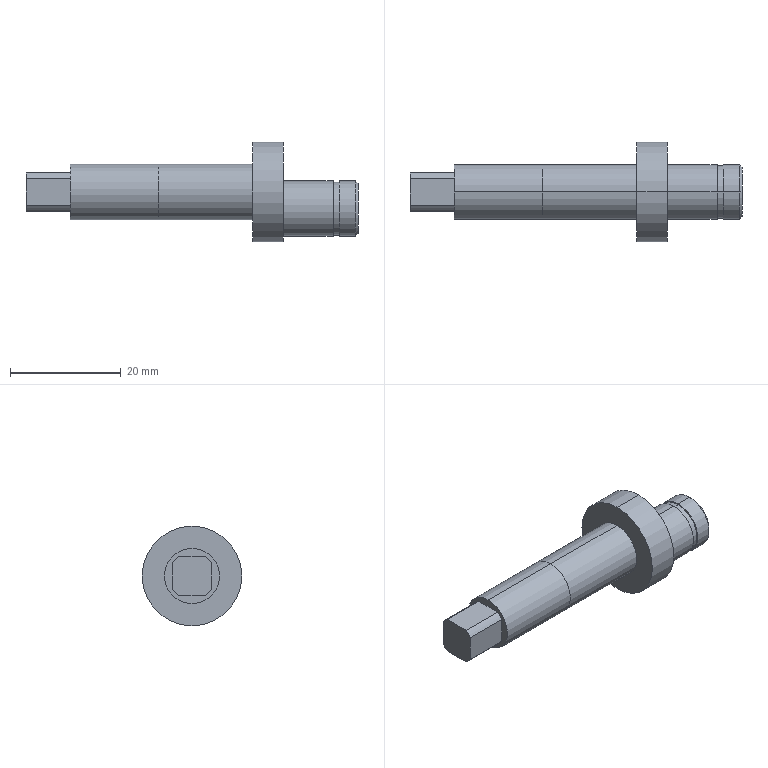Part | SolidWorks | features ICE 6, Chamfer 1, Extrusion 1 | 2 solids | 31 faces | box 60 x 18 x 18 mm | volume 5416 mm3 | cylinder 16 | plane 13 | cone 2 | commonest cylinder face diameters 10 x8 8.5 x4 9.6 x2 18 x2
STEP:
#1=CARTESIAN_POINT('',(-17.,0.,5.));
#2=VERTEX_POINT('',#1);
#3=CARTESIAN_POINT('',(-17.,0.,-5.));
#4=VERTEX_POINT('',#3);
#5=CARTESIAN_POINT('',(-17.,0.,0.));
#6=DIRECTION('',(-1.,0.,0.));
#7=DIRECTION('',(0.,0.,1.));
#8=AXIS2_PLACEMENT_3D('',#5,#6,#7);
#9=CIRCLE('',#8,5.);
#10=EDGE_CURVE('',#2,#4,#9,.T.);
#11=ORIENTED_EDGE('',*,*,#10,.F.);
#12=CARTESIAN_POINT('',(0.,0.,5.));
#13=VERTEX_POINT('',#12);
#14=CARTESIAN_POINT('',(-17.,0.,5.));
#15=DIRECTION('',(1.,0.,0.));
#16=VECTOR('',#15,1000.);
#17=LINE('',#14,#16);
#18=EDGE_CURVE('',#2,#13,#17,.T.);
#19=ORIENTED_EDGE('',*,*,#18,.T.);
#20=CARTESIAN_POINT('',(0.,0.,-5.));
#21=VERTEX_POINT('',#20);
#22=CARTESIAN_POINT('',(0.,0.,0.));
#23=DIRECTION('',(-1.,0.,0.));
#24=DIRECTION('',(0.,0.,1.));
#25=AXIS2_PLACEMENT_3D('',#22,#23,#24);
#26=CIRCLE('',#25,5.);
#27=EDGE_CURVE('',#13,#21,#26,.T.);
#28=ORIENTED_EDGE('',*,*,#27,.T.);
#29=CARTESIAN_POINT('',(-17.,0.,-5.));
#30=DIRECTION('',(1.,0.,0.));
#31=VECTOR('',#30,1000.);
#32=LINE('',#29,#31);
#33=EDGE_CURVE('',#4,#21,#32,.T.);
#34=ORIENTED_EDGE('',*,*,#33,.F.);
#35=EDGE_LOOP('',(#11,#19,#28,#34));
#36=FACE_OUTER_BOUND('',#35,.T.);
#37=CARTESIAN_POINT('',(-17.,0.,0.));
#38=DIRECTION('',(1.,0.,0.));
#39=DIRECTION('',(0.,0.,-1.));
#40=AXIS2_PLACEMENT_3D('',#37,#38,#39);
#41=CYLINDRICAL_SURFACE('',#40,5.);
#42=ADVANCED_FACE('',(#36),#41,.T.);
#43=CARTESIAN_POINT('',(19.,0.,-7.5));
#44=VERTEX_POINT('',#43);
#45=CARTESIAN_POINT('',(19.,0.,1.5));
#46=VERTEX_POINT('',#45);
#47=CARTESIAN_POINT('',(19.,0.,-3.));
#48=DIRECTION('',(1.,0.,0.));
#49=DIRECTION('',(0.,0.,-1.));
#50=AXIS2_PLACEMENT_3D('',#47,#48,#49);
#51=CIRCLE('',#50,4.5);
#52=EDGE_CURVE('',#44,#46,#51,.T.);
#53=ORIENTED_EDGE('',*,*,#52,.F.);
#54=CARTESIAN_POINT('',(18.5,0.,-8.));
#55=VERTEX_POINT('',#54);
#56=CARTESIAN_POINT('',(19.,0.,-7.5));
#57=DIRECTION('',(-0.7071,0.,-0.7071));
#58=VECTOR('',#57,1000.);
#59=LINE('',#56,#58);
#60=EDGE_CURVE('',#44,#55,#59,.T.);
#61=ORIENTED_EDGE('',*,*,#60,.T.);
#62=CARTESIAN_POINT('',(18.5,0.,2.));
#63=VERTEX_POINT('',#62);
#64=CARTESIAN_POINT('',(18.5,0.,-3.));
#65=DIRECTION('',(-1.,0.,0.));
#66=DIRECTION('',(0.,0.,-1.));
#67=AXIS2_PLACEMENT_3D('',#64,#65,#66);
#68=CIRCLE('',#67,5.);
#69=EDGE_CURVE('',#63,#55,#68,.T.);
#70=ORIENTED_EDGE('',*,*,#69,.F.);
#71=CARTESIAN_POINT('',(19.,0.,1.5));
#72=DIRECTION('',(-0.7071,0.,0.7071));
#73=VECTOR('',#72,1000.);
#74=LINE('',#71,#73);
#75=EDGE_CURVE('',#46,#63,#74,.T.);
#76=ORIENTED_EDGE('',*,*,#75,.F.);
#77=EDGE_LOOP('',(#53,#61,#70,#76));
#78=FACE_OUTER_BOUND('',#77,.T.);
#79=CARTESIAN_POINT('',(19.,0.,-3.));
#80=DIRECTION('',(-1.,0.,0.));
#81=DIRECTION('',(0.,0.,1.));
#82=AXIS2_PLACEMENT_3D('',#79,#80,#81);
#83=CONICAL_SURFACE('',#82,4.5,0.7854);
#84=ADVANCED_FACE('',(#78),#83,.T.);
#85=ORIENTED_EDGE('',*,*,#69,.T.);
#86=CARTESIAN_POINT('',(15.6,0.,-8.));
#87=VERTEX_POINT('',#86);
#88=CARTESIAN_POINT('',(19.,0.,-8.));
#89=DIRECTION('',(-1.,0.,0.));
#90=VECTOR('',#89,1000.);
#91=LINE('',#88,#90);
#92=EDGE_CURVE('',#55,#87,#91,.T.);
#93=ORIENTED_EDGE('',*,*,#92,.T.);
#94=CARTESIAN_POINT('',(15.6,0.,2.));
#95=VERTEX_POINT('',#94);
#96=CARTESIAN_POINT('',(15.6,0.,-3.));
#97=DIRECTION('',(1.,0.,0.));
#98=DIRECTION('',(0.,0.,-1.));
#99=AXIS2_PLACEMENT_3D('',#96,#97,#98);
#100=CIRCLE('',#99,5.);
#101=EDGE_CURVE('',#87,#95,#100,.T.);
#102=ORIENTED_EDGE('',*,*,#101,.T.);
#103=CARTESIAN_POINT('',(19.,0.,2.));
#104=DIRECTION('',(-1.,0.,0.));
#105=VECTOR('',#104,1000.);
#106=LINE('',#103,#105);
#107=EDGE_CURVE('',#63,#95,#106,.T.);
#108=ORIENTED_EDGE('',*,*,#107,.F.);
#109=EDGE_LOOP('',(#85,#93,#102,#108));
#110=FACE_OUTER_BOUND('',#109,.T.);
#111=CARTESIAN_POINT('',(19.,0.,-3.));
#112=DIRECTION('',(-1.,0.,0.));
#113=DIRECTION('',(0.,0.,1.));
#114=AXIS2_PLACEMENT_3D('',#111,#112,#113);
#115=CYLINDRICAL_SURFACE('',#114,5.);
#116=ADVANCED_FACE('',(#110),#115,.T.);
#117=CARTESIAN_POINT('',(15.6,0.,-7.8));
#118=VERTEX_POINT('',#117);
#119=CARTESIAN_POINT('',(15.6,0.,1.8));
#120=VERTEX_POINT('',#119);
#121=CARTESIAN_POINT('',(15.6,0.,-3.));
#122=DIRECTION('',(1.,0.,0.));
#123=DIRECTION('',(0.,0.,-1.));
#124=AXIS2_PLACEMENT_3D('',#121,#122,#123);
#125=CIRCLE('',#124,4.8);
#126=EDGE_CURVE('',#118,#120,#125,.T.);
#127=ORIENTED_EDGE('',*,*,#126,.F.);
#128=CARTESIAN_POINT('',(14.5,0.,-7.8));
#129=VERTEX_POINT('',#128);
#130=CARTESIAN_POINT('',(15.6,0.,-7.8));
#131=DIRECTION('',(-1.,0.,0.));
#132=VECTOR('',#131,1000.);
#133=LINE('',#130,#132);
#134=EDGE_CURVE('',#118,#129,#133,.T.);
#135=ORIENTED_EDGE('',*,*,#134,.T.);
#136=CARTESIAN_POINT('',(14.5,0.,1.8));
#137=VERTEX_POINT('',#136);
#138=CARTESIAN_POINT('',(14.5,0.,-3.));
#139=DIRECTION('',(1.,0.,0.));
#140=DIRECTION('',(0.,0.,-1.));
#141=AXIS2_PLACEMENT_3D('',#138,#139,#140);
#142=CIRCLE('',#141,4.8);
#143=EDGE_CURVE('',#129,#137,#142,.T.);
#144=ORIENTED_EDGE('',*,*,#143,.T.);
#145=CARTESIAN_POINT('',(15.6,0.,1.8));
#146=DIRECTION('',(-1.,0.,0.));
#147=VECTOR('',#146,1000.);
#148=LINE('',#145,#147);
#149=EDGE_CURVE('',#120,#137,#148,.T.);
#150=ORIENTED_EDGE('',*,*,#149,.F.);
#151=EDGE_LOOP('',(#127,#135,#144,#150));
#152=FACE_OUTER_BOUND('',#151,.T.);
#153=CARTESIAN_POINT('',(15.6,0.,-3.));
#154=DIRECTION('',(-1.,0.,0.));
#155=DIRECTION('',(0.,0.,1.));
#156=AXIS2_PLACEMENT_3D('',#153,#154,#155);
#157=CYLINDRICAL_SURFACE('',#156,4.8);
#158=ADVANCED_FACE('',(#152),#157,.T.);
#159=CARTESIAN_POINT('',(14.5,0.,-8.));
#160=VERTEX_POINT('',#159);
#161=CARTESIAN_POINT('',(14.5,0.,2.));
#162=VERTEX_POINT('',#161);
#163=CARTESIAN_POINT('',(14.5,0.,-3.));
#164=DIRECTION('',(1.,0.,0.));
#165=DIRECTION('',(0.,0.,-1.));
#166=AXIS2_PLACEMENT_3D('',#163,#164,#165);
#167=CIRCLE('',#166,5.);
#168=EDGE_CURVE('',#160,#162,#167,.T.);
#169=ORIENTED_EDGE('',*,*,#168,.F.);
#170=CARTESIAN_POINT('',(5.5,0.,-8.));
#171=VERTEX_POINT('',#170);
#172=CARTESIAN_POINT('',(14.5,0.,-8.));
#173=DIRECTION('',(-1.,0.,0.));
#174=VECTOR('',#173,1000.);
#175=LINE('',#172,#174);
#176=EDGE_CURVE('',#160,#171,#175,.T.);
#177=ORIENTED_EDGE('',*,*,#176,.T.);
#178=CARTESIAN_POINT('',(5.5,0.,2.));
#179=VERTEX_POINT('',#178);
#180=CARTESIAN_POINT('',(5.5,0.,-3.));
#181=DIRECTION('',(1.,0.,0.));
#182=DIRECTION('',(0.,0.,-1.));
#183=AXIS2_PLACEMENT_3D('',#180,#181,#182);
#184=CIRCLE('',#183,5.);
#185=EDGE_CURVE('',#171,#179,#184,.T.);
#186=ORIENTED_EDGE('',*,*,#185,.T.);
#187=CARTESIAN_POINT('',(14.5,0.,2.));
#188=DIRECTION('',(-1.,0.,0.));
#189=VECTOR('',#188,1000.);
#190=LINE('',#187,#189);
#191=EDGE_CURVE('',#162,#179,#190,.T.);
#192=ORIENTED_EDGE('',*,*,#191,.F.);
#193=EDGE_LOOP('',(#169,#177,#186,#192));
#194=FACE_OUTER_BOUND('',#193,.T.);
#195=CARTESIAN_POINT('',(14.5,0.,-3.));
#196=DIRECTION('',(-1.,0.,0.));
#197=DIRECTION('',(0.,0.,1.));
#198=AXIS2_PLACEMENT_3D('',#195,#196,#197);
#199=CYLINDRICAL_SURFACE('',#198,5.);
#200=ADVANCED_FACE('',(#194),#199,.T.);
#201=CARTESIAN_POINT('',(5.5,0.,-9.));
#202=VERTEX_POINT('',#201);
#203=CARTESIAN_POINT('',(5.5,0.,9.));
#204=VERTEX_POINT('',#203);
#205=CARTESIAN_POINT('',(5.5,0.,0.));
#206=DIRECTION('',(1.,0.,0.));
#207=DIRECTION('',(0.,0.,-1.));
#208=AXIS2_PLACEMENT_3D('',#205,#206,#207);
#209=CIRCLE('',#208,9.);
#210=EDGE_CURVE('',#202,#204,#209,.T.);
#211=ORIENTED_EDGE('',*,*,#210,.F.);
#212=CARTESIAN_POINT('',(0.,0.,-9.));
#213=VERTEX_POINT('',#212);
#214=CARTESIAN_POINT('',(5.5,0.,-9.));
#215=DIRECTION('',(-1.,0.,0.));
#216=VECTOR('',#215,1000.);
#217=LINE('',#214,#216);
#218=EDGE_CURVE('',#202,#213,#217,.T.);
#219=ORIENTED_EDGE('',*,*,#218,.T.);
#220=CARTESIAN_POINT('',(0.,0.,9.));
#221=VERTEX_POINT('',#220);
#222=CARTESIAN_POINT('',(0.,0.,0.));
#223=DIRECTION('',(1.,0.,0.));
#224=DIRECTION('',(0.,0.,-1.));
#225=AXIS2_PLACEMENT_3D('',#222,#223,#224);
#226=CIRCLE('',#225,9.);
#227=EDGE_CURVE('',#213,#221,#226,.T.);
#228=ORIENTED_EDGE('',*,*,#227,.T.);
#229=CARTESIAN_POINT('',(5.5,0.,9.));
#230=DIRECTION('',(-1.,0.,0.));
#231=VECTOR('',#230,1000.);
#232=LINE('',#229,#231);
#233=EDGE_CURVE('',#204,#221,#232,.T.);
#234=ORIENTED_EDGE('',*,*,#233,.F.);
#235=EDGE_LOOP('',(#211,#219,#228,#234));
#236=FACE_OUTER_BOUND('',#235,.T.);
#237=CARTESIAN_POINT('',(5.5,0.,0.));
#238=DIRECTION('',(-1.,0.,0.));
#239=DIRECTION('',(0.,0.,1.));
#240=AXIS2_PLACEMENT_3D('',#237,#238,#239);
#241=CYLINDRICAL_SURFACE('',#240,9.);
#242=ADVANCED_FACE('',(#236),#241,.T.);
#243=ORIENTED_EDGE('',*,*,#218,.F.);
#244=CARTESIAN_POINT('',(5.5,0.,0.));
#245=DIRECTION('',(1.,0.,0.));
#246=DIRECTION('',(0.,0.,-1.));
#247=AXIS2_PLACEMENT_3D('',#244,#245,#246);
#248=CIRCLE('',#247,9.);
#249=EDGE_CURVE('',#204,#202,#248,.T.);
#250=ORIENTED_EDGE('',*,*,#249,.F.);
#251=ORIENTED_EDGE('',*,*,#233,.T.);
#252=CARTESIAN_POINT('',(0.,0.,0.));
#253=DIRECTION('',(1.,0.,0.));
#254=DIRECTION('',(0.,0.,-1.));
#255=AXIS2_PLACEMENT_3D('',#252,#253,#254);
#256=CIRCLE('',#255,9.);
#257=EDGE_CURVE('',#221,#213,#256,.T.);
#258=ORIENTED_EDGE('',*,*,#257,.T.);
#259=EDGE_LOOP('',(#243,#250,#251,#258));
#260=FACE_OUTER_BOUND('',#259,.T.);
#261=CARTESIAN_POINT('',(5.5,0.,0.));
#262=DIRECTION('',(-1.,0.,0.));
#263=DIRECTION('',(0.,0.,1.));
#264=AXIS2_PLACEMENT_3D('',#261,#262,#263);
#265=CYLINDRICAL_SURFACE('',#264,9.);
#266=ADVANCED_FACE('',(#260),#265,.T.);
#267=CARTESIAN_POINT('',(5.5,0.,-3.));
#268=DIRECTION('',(1.,0.,0.));
#269=DIRECTION('',(0.,0.,-1.));
#270=AXIS2_PLACEMENT_3D('',#267,#268,#269);
#271=CIRCLE('',#270,5.);
#272=EDGE_CURVE('',#179,#171,#271,.T.);
#273=ORIENTED_EDGE('',*,*,#272,.F.);
#274=ORIENTED_EDGE('',*,*,#185,.F.);
#275=EDGE_LOOP('',(#273,#274));
#276=FACE_BOUND('',#275,.T.);
#277=ORIENTED_EDGE('',*,*,#249,.T.);
#278=ORIENTED_EDGE('',*,*,#210,.T.);
#279=EDGE_LOOP('',(#277,#278));
#280=FACE_OUTER_BOUND('',#279,.T.);
#281=CARTESIAN_POINT('',(5.5,0.,0.));
#282=DIRECTION('',(1.,0.,0.));
#283=DIRECTION('',(0.,0.,-1.));
#284=AXIS2_PLACEMENT_3D('',#281,#282,#283);
#285=PLANE('',#284);
#286=ADVANCED_FACE('',(#276,#280),#285,.T.);
#287=CARTESIAN_POINT('',(0.,0.,0.));
#288=DIRECTION('',(-1.,0.,0.));
#289=DIRECTION('',(0.,0.,1.));
#290=AXIS2_PLACEMENT_3D('',#287,#288,#289);
#291=CIRCLE('',#290,5.);
#292=EDGE_CURVE('',#21,#13,#291,.T.);
#293=ORIENTED_EDGE('',*,*,#292,.F.);
#294=ORIENTED_EDGE('',*,*,#27,.F.);
#295=EDGE_LOOP('',(#293,#294));
#296=FACE_BOUND('',#295,.T.);
#297=ORIENTED_EDGE('',*,*,#257,.F.);
#298=ORIENTED_EDGE('',*,*,#227,.F.);
#299=EDGE_LOOP('',(#297,#298));
#300=FACE_OUTER_BOUND('',#299,.T.);
#301=CARTESIAN_POINT('',(0.,0.,0.));
#302=DIRECTION('',(1.,0.,0.));
#303=DIRECTION('',(0.,0.,-1.));
#304=AXIS2_PLACEMENT_3D('',#301,#302,#303);
#305=PLANE('',#304);
#306=ADVANCED_FACE('',(#296,#300),#305,.F.);
#307=ORIENTED_EDGE('',*,*,#176,.F.);
#308=CARTESIAN_POINT('',(14.5,0.,-3.));
#309=DIRECTION('',(1.,0.,0.));
#310=DIRECTION('',(0.,0.,-1.));
#311=AXIS2_PLACEMENT_3D('',#308,#309,#310);
#312=CIRCLE('',#311,5.);
#313=EDGE_CURVE('',#162,#160,#312,.T.);
#314=ORIENTED_EDGE('',*,*,#313,.F.);
#315=ORIENTED_EDGE('',*,*,#191,.T.);
#316=ORIENTED_EDGE('',*,*,#272,.T.);
#317=EDGE_LOOP('',(#307,#314,#315,#316));
#318=FACE_OUTER_BOUND('',#317,.T.);
#319=CARTESIAN_POINT('',(14.5,0.,-3.));
#320=DIRECTION('',(-1.,0.,0.));
#321=DIRECTION('',(0.,0.,1.));
#322=AXIS2_PLACEMENT_3D('',#319,#320,#321);
#323=CYLINDRICAL_SURFACE('',#322,5.);
#324=ADVANCED_FACE('',(#318),#323,.T.);
#325=CARTESIAN_POINT('',(14.5,0.,-3.));
#326=DIRECTION('',(1.,0.,0.));
#327=DIRECTION('',(0.,0.,-1.));
#328=AXIS2_PLACEMENT_3D('',#325,#326,#327);
#329=CIRCLE('',#328,4.8);
#330=EDGE_CURVE('',#137,#129,#329,.T.);
#331=ORIENTED_EDGE('',*,*,#330,.F.);
#332=ORIENTED_EDGE('',*,*,#143,.F.);
#333=EDGE_LOOP('',(#331,#332));
#334=FACE_BOUND('',#333,.T.);
#335=ORIENTED_EDGE('',*,*,#313,.T.);
#336=ORIENTED_EDGE('',*,*,#168,.T.);
#337=EDGE_LOOP('',(#335,#336));
#338=FACE_OUTER_BOUND('',#337,.T.);
#339=CARTESIAN_POINT('',(14.5,0.,-3.));
#340=DIRECTION('',(1.,0.,0.));
#341=DIRECTION('',(0.,0.,-1.));
#342=AXIS2_PLACEMENT_3D('',#339,#340,#341);
#343=PLANE('',#342);
#344=ADVANCED_FACE('',(#334,#338),#343,.T.);
#345=ORIENTED_EDGE('',*,*,#134,.F.);
#346=CARTESIAN_POINT('',(15.6,0.,-3.));
#347=DIRECTION('',(1.,0.,0.));
#348=DIRECTION('',(0.,0.,-1.));
#349=AXIS2_PLACEMENT_3D('',#346,#347,#348);
#350=CIRCLE('',#349,4.8);
#351=EDGE_CURVE('',#120,#118,#350,.T.);
#352=ORIENTED_EDGE('',*,*,#351,.F.);
#353=ORIENTED_EDGE('',*,*,#149,.T.);
#354=ORIENTED_EDGE('',*,*,#330,.T.);
#355=EDGE_LOOP('',(#345,#352,#353,#354));
#356=FACE_OUTER_BOUND('',#355,.T.);
#357=CARTESIAN_POINT('',(15.6,0.,-3.));
#358=DIRECTION('',(-1.,0.,0.));
#359=DIRECTION('',(0.,0.,1.));
#360=AXIS2_PLACEMENT_3D('',#357,#358,#359);
#361=CYLINDRICAL_SURFACE('',#360,4.8);
#362=ADVANCED_FACE('',(#356),#361,.T.);
#363=ORIENTED_EDGE('',*,*,#92,.F.);
#364=CARTESIAN_POINT('',(18.5,0.,-3.));
#365=DIRECTION('',(-1.,0.,0.));
#366=DIRECTION('',(0.,0.,-1.));
#367=AXIS2_PLACEMENT_3D('',#364,#365,#366);
#368=CIRCLE('',#367,5.);
#369=EDGE_CURVE('',#55,#63,#368,.T.);
#370=ORIENTED_EDGE('',*,*,#369,.T.);
#371=ORIENTED_EDGE('',*,*,#107,.T.);
#372=CARTESIAN_POINT('',(15.6,0.,-3.));
#373=DIRECTION('',(1.,0.,0.));
#374=DIRECTION('',(0.,0.,-1.));
#375=AXIS2_PLACEMENT_3D('',#372,#373,#374);
#376=CIRCLE('',#375,5.);
#377=EDGE_CURVE('',#95,#87,#376,.T.);
#378=ORIENTED_EDGE('',*,*,#377,.T.);
#379=EDGE_LOOP('',(#363,#370,#371,#378));
#380=FACE_OUTER_BOUND('',#379,.T.);
#381=CARTESIAN_POINT('',(19.,0.,-3.));
#382=DIRECTION('',(-1.,0.,0.));
#383=DIRECTION('',(0.,0.,1.));
#384=AXIS2_PLACEMENT_3D('',#381,#382,#383);
#385=CYLINDRICAL_SURFACE('',#384,5.);
#386=ADVANCED_FACE('',(#380),#385,.T.);
#387=CARTESIAN_POINT('',(19.,0.,-3.));
#388=DIRECTION('',(1.,0.,0.));
#389=DIRECTION('',(0.,0.,-1.));
#390=AXIS2_PLACEMENT_3D('',#387,#388,#389);
#391=CIRCLE('',#390,4.5);
#392=EDGE_CURVE('',#46,#44,#391,.T.);
#393=ORIENTED_EDGE('',*,*,#392,.T.);
#394=ORIENTED_EDGE('',*,*,#52,.T.);
#395=EDGE_LOOP('',(#393,#394));
#396=FACE_OUTER_BOUND('',#395,.T.);
#397=CARTESIAN_POINT('',(19.,0.,-3.));
#398=DIRECTION('',(1.,0.,0.));
#399=DIRECTION('',(0.,0.,-1.));
#400=AXIS2_PLACEMENT_3D('',#397,#398,#399);
#401=PLANE('',#400);
#402=ADVANCED_FACE('',(#396),#401,.T.);
#403=ORIENTED_EDGE('',*,*,#351,.T.);
#404=ORIENTED_EDGE('',*,*,#126,.T.);
#405=EDGE_LOOP('',(#403,#404));
#406=FACE_BOUND('',#405,.T.);
#407=ORIENTED_EDGE('',*,*,#377,.F.);
#408=ORIENTED_EDGE('',*,*,#101,.F.);
#409=EDGE_LOOP('',(#407,#408));
#410=FACE_OUTER_BOUND('',#409,.T.);
#411=CARTESIAN_POINT('',(15.6,0.,-3.));
#412=DIRECTION('',(1.,0.,0.));
#413=DIRECTION('',(0.,0.,-1.));
#414=AXIS2_PLACEMENT_3D('',#411,#412,#413);
#415=PLANE('',#414);
#416=ADVANCED_FACE('',(#406,#410),#415,.F.);
#417=ORIENTED_EDGE('',*,*,#60,.F.);
#418=ORIENTED_EDGE('',*,*,#392,.F.);
#419=ORIENTED_EDGE('',*,*,#75,.T.);
#420=ORIENTED_EDGE('',*,*,#369,.F.);
#421=EDGE_LOOP('',(#417,#418,#419,#420));
#422=FACE_OUTER_BOUND('',#421,.T.);
#423=CARTESIAN_POINT('',(19.,0.,-3.));
#424=DIRECTION('',(-1.,0.,0.));
#425=DIRECTION('',(0.,0.,1.));
#426=AXIS2_PLACEMENT_3D('',#423,#424,#425);
#427=CONICAL_SURFACE('',#426,4.5,0.7854);
#428=ADVANCED_FACE('',(#422),#427,.T.);
#429=ORIENTED_EDGE('',*,*,#18,.F.);
#430=CARTESIAN_POINT('',(-17.,0.,0.));
#431=DIRECTION('',(-1.,0.,0.));
#432=DIRECTION('',(0.,0.,1.));
#433=AXIS2_PLACEMENT_3D('',#430,#431,#432);
#434=CIRCLE('',#433,5.);
#435=EDGE_CURVE('',#4,#2,#434,.T.);
#436=ORIENTED_EDGE('',*,*,#435,.F.);
#437=ORIENTED_EDGE('',*,*,#33,.T.);
#438=ORIENTED_EDGE('',*,*,#292,.T.);
#439=EDGE_LOOP('',(#429,#436,#437,#438));
#440=FACE_OUTER_BOUND('',#439,.T.);
#441=CARTESIAN_POINT('',(-17.,0.,0.));
#442=DIRECTION('',(1.,0.,0.));
#443=DIRECTION('',(0.,0.,-1.));
#444=AXIS2_PLACEMENT_3D('',#441,#442,#443);
#445=CYLINDRICAL_SURFACE('',#444,5.);
#446=ADVANCED_FACE('',(#440),#445,.T.);
#447=ORIENTED_EDGE('',*,*,#435,.T.);
#448=ORIENTED_EDGE('',*,*,#10,.T.);
#449=EDGE_LOOP('',(#447,#448));
#450=FACE_OUTER_BOUND('',#449,.T.);
#451=CARTESIAN_POINT('',(-17.,0.,0.));
#452=DIRECTION('',(-1.,0.,0.));
#453=DIRECTION('',(0.,0.,1.));
#454=AXIS2_PLACEMENT_3D('',#451,#452,#453);
#455=PLANE('',#454);
#456=ADVANCED_FACE('',(#450),#455,.T.);
#457=CLOSED_SHELL('',(#42,#84,#116,#158,#200,#242,#266,#286,#306,#324,#344,#362,#386,#402,#416,#428,#446,#456));
#458=MANIFOLD_SOLID_BREP('',#457);
#459=CARTESIAN_POINT('',(-33.,0.,5.));
#460=VERTEX_POINT('',#459);
#461=CARTESIAN_POINT('',(-33.,0.,-5.));
#462=VERTEX_POINT('',#461);
#463=CARTESIAN_POINT('',(-33.,0.,0.));
#464=DIRECTION('',(-1.,0.,0.));
#465=DIRECTION('',(0.,0.,1.));
#466=AXIS2_PLACEMENT_3D('',#463,#464,#465);
#467=CIRCLE('',#466,5.);
#468=EDGE_CURVE('',#460,#462,#467,.T.);
#469=ORIENTED_EDGE('',*,*,#468,.F.);
#470=CARTESIAN_POINT('',(-17.,0.,5.));
#471=VERTEX_POINT('',#470);
#472=CARTESIAN_POINT('',(-33.,0.,5.));
#473=DIRECTION('',(1.,0.,0.));
#474=VECTOR('',#473,1000.);
#475=LINE('',#472,#474);
#476=EDGE_CURVE('',#460,#471,#475,.T.);
#477=ORIENTED_EDGE('',*,*,#476,.T.);
#478=CARTESIAN_POINT('',(-17.,0.,-5.));
#479=VERTEX_POINT('',#478);
#480=CARTESIAN_POINT('',(-17.,0.,0.));
#481=DIRECTION('',(-1.,0.,0.));
#482=DIRECTION('',(0.,0.,1.));
#483=AXIS2_PLACEMENT_3D('',#480,#481,#482);
#484=CIRCLE('',#483,5.);
#485=EDGE_CURVE('',#471,#479,#484,.T.);
#486=ORIENTED_EDGE('',*,*,#485,.T.);
#487=CARTESIAN_POINT('',(-33.,0.,-5.));
#488=DIRECTION('',(1.,0.,0.));
#489=VECTOR('',#488,1000.);
#490=LINE('',#487,#489);
#491=EDGE_CURVE('',#462,#479,#490,.T.);
#492=ORIENTED_EDGE('',*,*,#491,.F.);
#493=EDGE_LOOP('',(#469,#477,#486,#492));
#494=FACE_OUTER_BOUND('',#493,.T.);
#495=CARTESIAN_POINT('',(-33.,0.,0.));
#496=DIRECTION('',(1.,0.,0.));
#497=DIRECTION('',(0.,0.,-1.));
#498=AXIS2_PLACEMENT_3D('',#495,#496,#497);
#499=CYLINDRICAL_SURFACE('',#498,5.);
#500=ADVANCED_FACE('',(#494),#499,.T.);
#501=ORIENTED_EDGE('',*,*,#476,.F.);
#502=CARTESIAN_POINT('',(-33.,0.,0.));
#503=DIRECTION('',(-1.,0.,0.));
#504=DIRECTION('',(0.,0.,1.));
#505=AXIS2_PLACEMENT_3D('',#502,#503,#504);
#506=CIRCLE('',#505,5.);
#507=EDGE_CURVE('',#462,#460,#506,.T.);
#508=ORIENTED_EDGE('',*,*,#507,.F.);
#509=ORIENTED_EDGE('',*,*,#491,.T.);
#510=CARTESIAN_POINT('',(-17.,0.,0.));
#511=DIRECTION('',(-1.,0.,0.));
#512=DIRECTION('',(0.,0.,1.));
#513=AXIS2_PLACEMENT_3D('',#510,#511,#512);
#514=CIRCLE('',#513,5.);
#515=EDGE_CURVE('',#479,#471,#514,.T.);
#516=ORIENTED_EDGE('',*,*,#515,.T.);
#517=EDGE_LOOP('',(#501,#508,#509,#516));
#518=FACE_OUTER_BOUND('',#517,.T.);
#519=CARTESIAN_POINT('',(-33.,0.,0.));
#520=DIRECTION('',(1.,0.,0.));
#521=DIRECTION('',(0.,0.,-1.));
#522=AXIS2_PLACEMENT_3D('',#519,#520,#521);
#523=CYLINDRICAL_SURFACE('',#522,5.);
#524=ADVANCED_FACE('',(#518),#523,.T.);
#525=CARTESIAN_POINT('',(-33.,3.5,-2.411));
#526=VERTEX_POINT('',#525);
#527=CARTESIAN_POINT('',(-33.,2.411,-3.5));
#528=VERTEX_POINT('',#527);
#529=CARTESIAN_POINT('',(-33.,0.,0.));
#530=DIRECTION('',(-1.,0.,0.));
#531=DIRECTION('',(0.,0.,1.));
#532=AXIS2_PLACEMENT_3D('',#529,#530,#531);
#533=CIRCLE('',#532,4.25);
#534=EDGE_CURVE('',#526,#528,#533,.T.);
#535=ORIENTED_EDGE('',*,*,#534,.F.);
#536=CARTESIAN_POINT('',(-33.,3.5,2.411));
#537=VERTEX_POINT('',#536);
#538=CARTESIAN_POINT('',(-33.,3.5,-2.411));
#539=DIRECTION('',(0.,0.,-1.));
#540=VECTOR('',#539,1000.);
#541=LINE('',#538,#540);
#542=EDGE_CURVE('',#537,#526,#541,.T.);
#543=ORIENTED_EDGE('',*,*,#542,.F.);
#544=CARTESIAN_POINT('',(-33.,2.411,3.5));
#545=VERTEX_POINT('',#544);
#546=CARTESIAN_POINT('',(-33.,0.,0.));
#547=DIRECTION('',(-1.,0.,0.));
#548=DIRECTION('',(0.,0.,1.));
#549=AXIS2_PLACEMENT_3D('',#546,#547,#548);
#550=CIRCLE('',#549,4.25);
#551=EDGE_CURVE('',#545,#537,#550,.T.);
#552=ORIENTED_EDGE('',*,*,#551,.F.);
#553=CARTESIAN_POINT('',(-33.,-2.411,3.5));
#554=VERTEX_POINT('',#553);
#555=CARTESIAN_POINT('',(-33.,-2.411,3.5));
#556=DIRECTION('',(0.,1.,0.));
#557=VECTOR('',#556,1000.);
#558=LINE('',#555,#557);
#559=EDGE_CURVE('',#554,#545,#558,.T.);
#560=ORIENTED_EDGE('',*,*,#559,.F.);
#561=CARTESIAN_POINT('',(-33.,-3.5,2.411));
#562=VERTEX_POINT('',#561);
#563=CARTESIAN_POINT('',(-33.,0.,0.));
#564=DIRECTION('',(-1.,0.,0.));
#565=DIRECTION('',(0.,0.,1.));
#566=AXIS2_PLACEMENT_3D('',#563,#564,#565);
#567=CIRCLE('',#566,4.25);
#568=EDGE_CURVE('',#562,#554,#567,.T.);
#569=ORIENTED_EDGE('',*,*,#568,.F.);
#570=CARTESIAN_POINT('',(-33.,-3.5,-2.411));
#571=VERTEX_POINT('',#570);
#572=CARTESIAN_POINT('',(-33.,-3.5,-2.411));
#573=DIRECTION('',(0.,0.,1.));
#574=VECTOR('',#573,1000.);
#575=LINE('',#572,#574);
#576=EDGE_CURVE('',#571,#562,#575,.T.);
#577=ORIENTED_EDGE('',*,*,#576,.F.);
#578=CARTESIAN_POINT('',(-33.,-2.411,-3.5));
#579=VERTEX_POINT('',#578);
#580=CARTESIAN_POINT('',(-33.,0.,0.));
#581=DIRECTION('',(-1.,0.,0.));
#582=DIRECTION('',(0.,0.,1.));
#583=AXIS2_PLACEMENT_3D('',#580,#581,#582);
#584=CIRCLE('',#583,4.25);
#585=EDGE_CURVE('',#579,#571,#584,.T.);
#586=ORIENTED_EDGE('',*,*,#585,.F.);
#587=CARTESIAN_POINT('',(-33.,-2.411,-3.5));
#588=DIRECTION('',(0.,-1.,0.));
#589=VECTOR('',#588,1000.);
#590=LINE('',#587,#589);
#591=EDGE_CURVE('',#528,#579,#590,.T.);
#592=ORIENTED_EDGE('',*,*,#591,.F.);
#593=EDGE_LOOP('',(#535,#543,#552,#560,#569,#577,#586,#592));
#594=FACE_BOUND('',#593,.T.);
#595=ORIENTED_EDGE('',*,*,#507,.T.);
#596=ORIENTED_EDGE('',*,*,#468,.T.);
#597=EDGE_LOOP('',(#595,#596));
#598=FACE_OUTER_BOUND('',#597,.T.);
#599=CARTESIAN_POINT('',(-33.,0.,0.));
#600=DIRECTION('',(-1.,0.,0.));
#601=DIRECTION('',(0.,0.,1.));
#602=AXIS2_PLACEMENT_3D('',#599,#600,#601);
#603=PLANE('',#602);
#604=ADVANCED_FACE('',(#594,#598),#603,.T.);
#605=ORIENTED_EDGE('',*,*,#515,.F.);
#606=ORIENTED_EDGE('',*,*,#485,.F.);
#607=EDGE_LOOP('',(#605,#606));
#608=FACE_OUTER_BOUND('',#607,.T.);
#609=CARTESIAN_POINT('',(-17.,0.,0.));
#610=DIRECTION('',(-1.,0.,0.));
#611=DIRECTION('',(0.,0.,1.));
#612=AXIS2_PLACEMENT_3D('',#609,#610,#611);
#613=PLANE('',#612);
#614=ADVANCED_FACE('',(#608),#613,.F.);
#615=ORIENTED_EDGE('',*,*,#534,.T.);
#616=CARTESIAN_POINT('',(-41.,2.411,-3.5));
#617=VERTEX_POINT('',#616);
#618=CARTESIAN_POINT('',(-41.,2.411,-3.5));
#619=DIRECTION('',(1.,0.,0.));
#620=VECTOR('',#619,1000.);
#621=LINE('',#618,#620);
#622=EDGE_CURVE('',#617,#528,#621,.T.);
#623=ORIENTED_EDGE('',*,*,#622,.F.);
#624=CARTESIAN_POINT('',(-41.,3.5,-2.411));
#625=VERTEX_POINT('',#624);
#626=CARTESIAN_POINT('',(-41.,0.,0.));
#627=DIRECTION('',(-1.,0.,0.));
#628=DIRECTION('',(0.,0.,1.));
#629=AXIS2_PLACEMENT_3D('',#626,#627,#628);
#630=CIRCLE('',#629,4.25);
#631=EDGE_CURVE('',#625,#617,#630,.T.);
#632=ORIENTED_EDGE('',*,*,#631,.F.);
#633=CARTESIAN_POINT('',(-41.,3.5,-2.411));
#634=DIRECTION('',(1.,0.,0.));
#635=VECTOR('',#634,1000.);
#636=LINE('',#633,#635);
#637=EDGE_CURVE('',#625,#526,#636,.T.);
#638=ORIENTED_EDGE('',*,*,#637,.T.);
#639=EDGE_LOOP('',(#615,#623,#632,#638));
#640=FACE_OUTER_BOUND('',#639,.T.);
#641=CARTESIAN_POINT('',(-41.,0.,0.));
#642=DIRECTION('',(1.,0.,0.));
#643=DIRECTION('',(0.,0.,-1.));
#644=AXIS2_PLACEMENT_3D('',#641,#642,#643);
#645=CYLINDRICAL_SURFACE('',#644,4.25);
#646=ADVANCED_FACE('',(#640),#645,.T.);
#647=ORIENTED_EDGE('',*,*,#591,.T.);
#648=CARTESIAN_POINT('',(-41.,-2.411,-3.5));
#649=VERTEX_POINT('',#648);
#650=CARTESIAN_POINT('',(-41.,-2.411,-3.5));
#651=DIRECTION('',(1.,0.,0.));
#652=VECTOR('',#651,1000.);
#653=LINE('',#650,#652);
#654=EDGE_CURVE('',#649,#579,#653,.T.);
#655=ORIENTED_EDGE('',*,*,#654,.F.);
#656=CARTESIAN_POINT('',(-41.,-2.411,-3.5));
#657=DIRECTION('',(0.,-1.,0.));
#658=VECTOR('',#657,1000.);
#659=LINE('',#656,#658);
#660=EDGE_CURVE('',#617,#649,#659,.T.);
#661=ORIENTED_EDGE('',*,*,#660,.F.);
#662=ORIENTED_EDGE('',*,*,#622,.T.);
#663=EDGE_LOOP('',(#647,#655,#661,#662));
#664=FACE_OUTER_BOUND('',#663,.T.);
#665=CARTESIAN_POINT('',(-41.,-2.411,-3.5));
#666=DIRECTION('',(0.,0.,1.));
#667=DIRECTION('',(1.,0.,0.));
#668=AXIS2_PLACEMENT_3D('',#665,#666,#667);
#669=PLANE('',#668);
#670=ADVANCED_FACE('',(#664),#669,.F.);
#671=ORIENTED_EDGE('',*,*,#585,.T.);
#672=CARTESIAN_POINT('',(-41.,-3.5,-2.411));
#673=VERTEX_POINT('',#672);
#674=CARTESIAN_POINT('',(-41.,-3.5,-2.411));
#675=DIRECTION('',(1.,0.,0.));
#676=VECTOR('',#675,1000.);
#677=LINE('',#674,#676);
#678=EDGE_CURVE('',#673,#571,#677,.T.);
#679=ORIENTED_EDGE('',*,*,#678,.F.);
#680=CARTESIAN_POINT('',(-41.,0.,0.));
#681=DIRECTION('',(-1.,0.,0.));
#682=DIRECTION('',(0.,0.,1.));
#683=AXIS2_PLACEMENT_3D('',#680,#681,#682);
#684=CIRCLE('',#683,4.25);
#685=EDGE_CURVE('',#649,#673,#684,.T.);
#686=ORIENTED_EDGE('',*,*,#685,.F.);
#687=ORIENTED_EDGE('',*,*,#654,.T.);
#688=EDGE_LOOP('',(#671,#679,#686,#687));
#689=FACE_OUTER_BOUND('',#688,.T.);
#690=CARTESIAN_POINT('',(-41.,0.,0.));
#691=DIRECTION('',(1.,0.,0.));
#692=DIRECTION('',(0.,0.,-1.));
#693=AXIS2_PLACEMENT_3D('',#690,#691,#692);
#694=CYLINDRICAL_SURFACE('',#693,4.25);
#695=ADVANCED_FACE('',(#689),#694,.T.);
#696=ORIENTED_EDGE('',*,*,#576,.T.);
#697=CARTESIAN_POINT('',(-41.,-3.5,2.411));
#698=VERTEX_POINT('',#697);
#699=CARTESIAN_POINT('',(-41.,-3.5,2.411));
#700=DIRECTION('',(1.,0.,0.));
#701=VECTOR('',#700,1000.);
#702=LINE('',#699,#701);
#703=EDGE_CURVE('',#698,#562,#702,.T.);
#704=ORIENTED_EDGE('',*,*,#703,.F.);
#705=CARTESIAN_POINT('',(-41.,-3.5,-2.411));
#706=DIRECTION('',(0.,0.,1.));
#707=VECTOR('',#706,1000.);
#708=LINE('',#705,#707);
#709=EDGE_CURVE('',#673,#698,#708,.T.);
#710=ORIENTED_EDGE('',*,*,#709,.F.);
#711=ORIENTED_EDGE('',*,*,#678,.T.);
#712=EDGE_LOOP('',(#696,#704,#710,#711));
#713=FACE_OUTER_BOUND('',#712,.T.);
#714=CARTESIAN_POINT('',(-41.,-3.5,-2.411));
#715=DIRECTION('',(0.,1.,0.));
#716=DIRECTION('',(0.,0.,1.));
#717=AXIS2_PLACEMENT_3D('',#714,#715,#716);
#718=PLANE('',#717);
#719=ADVANCED_FACE('',(#713),#718,.F.);
#720=ORIENTED_EDGE('',*,*,#568,.T.);
#721=CARTESIAN_POINT('',(-41.,-2.411,3.5));
#722=VERTEX_POINT('',#721);
#723=CARTESIAN_POINT('',(-41.,-2.411,3.5));
#724=DIRECTION('',(1.,0.,0.));
#725=VECTOR('',#724,1000.);
#726=LINE('',#723,#725);
#727=EDGE_CURVE('',#722,#554,#726,.T.);
#728=ORIENTED_EDGE('',*,*,#727,.F.);
#729=CARTESIAN_POINT('',(-41.,0.,0.));
#730=DIRECTION('',(-1.,0.,0.));
#731=DIRECTION('',(0.,0.,1.));
#732=AXIS2_PLACEMENT_3D('',#729,#730,#731);
#733=CIRCLE('',#732,4.25);
#734=EDGE_CURVE('',#698,#722,#733,.T.);
#735=ORIENTED_EDGE('',*,*,#734,.F.);
#736=ORIENTED_EDGE('',*,*,#703,.T.);
#737=EDGE_LOOP('',(#720,#728,#735,#736));
#738=FACE_OUTER_BOUND('',#737,.T.);
#739=CARTESIAN_POINT('',(-41.,0.,0.));
#740=DIRECTION('',(1.,0.,0.));
#741=DIRECTION('',(0.,0.,-1.));
#742=AXIS2_PLACEMENT_3D('',#739,#740,#741);
#743=CYLINDRICAL_SURFACE('',#742,4.25);
#744=ADVANCED_FACE('',(#738),#743,.T.);
#745=ORIENTED_EDGE('',*,*,#559,.T.);
#746=CARTESIAN_POINT('',(-41.,2.411,3.5));
#747=VERTEX_POINT('',#746);
#748=CARTESIAN_POINT('',(-41.,2.411,3.5));
#749=DIRECTION('',(1.,0.,0.));
#750=VECTOR('',#749,1000.);
#751=LINE('',#748,#750);
#752=EDGE_CURVE('',#747,#545,#751,.T.);
#753=ORIENTED_EDGE('',*,*,#752,.F.);
#754=CARTESIAN_POINT('',(-41.,-2.411,3.5));
#755=DIRECTION('',(0.,1.,0.));
#756=VECTOR('',#755,1000.);
#757=LINE('',#754,#756);
#758=EDGE_CURVE('',#722,#747,#757,.T.);
#759=ORIENTED_EDGE('',*,*,#758,.F.);
#760=ORIENTED_EDGE('',*,*,#727,.T.);
#761=EDGE_LOOP('',(#745,#753,#759,#760));
#762=FACE_OUTER_BOUND('',#761,.T.);
#763=CARTESIAN_POINT('',(-41.,-2.411,3.5));
#764=DIRECTION('',(0.,0.,-1.));
#765=DIRECTION('',(-1.,0.,0.));
#766=AXIS2_PLACEMENT_3D('',#763,#764,#765);
#767=PLANE('',#766);
#768=ADVANCED_FACE('',(#762),#767,.F.);
#769=ORIENTED_EDGE('',*,*,#551,.T.);
#770=CARTESIAN_POINT('',(-41.,3.5,2.411));
#771=VERTEX_POINT('',#770);
#772=CARTESIAN_POINT('',(-41.,3.5,2.411));
#773=DIRECTION('',(1.,0.,0.));
#774=VECTOR('',#773,1000.);
#775=LINE('',#772,#774);
#776=EDGE_CURVE('',#771,#537,#775,.T.);
#777=ORIENTED_EDGE('',*,*,#776,.F.);
#778=CARTESIAN_POINT('',(-41.,0.,0.));
#779=DIRECTION('',(-1.,0.,0.));
#780=DIRECTION('',(0.,0.,1.));
#781=AXIS2_PLACEMENT_3D('',#778,#779,#780);
#782=CIRCLE('',#781,4.25);
#783=EDGE_CURVE('',#747,#771,#782,.T.);
#784=ORIENTED_EDGE('',*,*,#783,.F.);
#785=ORIENTED_EDGE('',*,*,#752,.T.);
#786=EDGE_LOOP('',(#769,#777,#784,#785));
#787=FACE_OUTER_BOUND('',#786,.T.);
#788=CARTESIAN_POINT('',(-41.,0.,0.));
#789=DIRECTION('',(1.,0.,0.));
#790=DIRECTION('',(0.,0.,-1.));
#791=AXIS2_PLACEMENT_3D('',#788,#789,#790);
#792=CYLINDRICAL_SURFACE('',#791,4.25);
#793=ADVANCED_FACE('',(#787),#792,.T.);
#794=ORIENTED_EDGE('',*,*,#542,.T.);
#795=ORIENTED_EDGE('',*,*,#637,.F.);
#796=CARTESIAN_POINT('',(-41.,3.5,-2.411));
#797=DIRECTION('',(0.,0.,-1.));
#798=VECTOR('',#797,1000.);
#799=LINE('',#796,#798);
#800=EDGE_CURVE('',#771,#625,#799,.T.);
#801=ORIENTED_EDGE('',*,*,#800,.F.);
#802=ORIENTED_EDGE('',*,*,#776,.T.);
#803=EDGE_LOOP('',(#794,#795,#801,#802));
#804=FACE_OUTER_BOUND('',#803,.T.);
#805=CARTESIAN_POINT('',(-41.,3.5,-2.411));
#806=DIRECTION('',(0.,-1.,0.));
#807=DIRECTION('',(0.,0.,-1.));
#808=AXIS2_PLACEMENT_3D('',#805,#806,#807);
#809=PLANE('',#808);
#810=ADVANCED_FACE('',(#804),#809,.F.);
#811=ORIENTED_EDGE('',*,*,#631,.T.);
#812=ORIENTED_EDGE('',*,*,#660,.T.);
#813=ORIENTED_EDGE('',*,*,#685,.T.);
#814=ORIENTED_EDGE('',*,*,#709,.T.);
#815=ORIENTED_EDGE('',*,*,#734,.T.);
#816=ORIENTED_EDGE('',*,*,#758,.T.);
#817=ORIENTED_EDGE('',*,*,#783,.T.);
#818=ORIENTED_EDGE('',*,*,#800,.T.);
#819=EDGE_LOOP('',(#811,#812,#813,#814,#815,#816,#817,#818));
#820=FACE_OUTER_BOUND('',#819,.T.);
#821=CARTESIAN_POINT('',(-41.,0.,0.));
#822=DIRECTION('',(-1.,0.,0.));
#823=DIRECTION('',(0.,0.,1.));
#824=AXIS2_PLACEMENT_3D('',#821,#822,#823);
#825=PLANE('',#824);
#826=ADVANCED_FACE('',(#820),#825,.T.);
#827=CLOSED_SHELL('',(#500,#524,#604,#614,#646,#670,#695,#719,#744,#768,#793,#810,#826));
#828=MANIFOLD_SOLID_BREP('',#827);
#829=CARTESIAN_POINT('',(0.,0.,0.));
#830=DIRECTION('',(0.,0.,1.));
#831=DIRECTION('',(1.,0.,0.));
#832=AXIS2_PLACEMENT_3D('',#829,#830,#831);
#833=(LENGTH_UNIT()NAMED_UNIT(*)SI_UNIT(.MILLI.,.METRE.));
#834=UNCERTAINTY_MEASURE_WITH_UNIT(LENGTH_MEASURE(0.00001),#833,'','');
#835=(NAMED_UNIT(*)PLANE_ANGLE_UNIT()SI_UNIT($,.RADIAN.));
#836=(NAMED_UNIT(*)SI_UNIT($,.STERADIAN.)SOLID_ANGLE_UNIT());
#837=(GEOMETRIC_REPRESENTATION_CONTEXT(3)GLOBAL_UNCERTAINTY_ASSIGNED_CONTEXT((#834))GLOBAL_UNIT_ASSIGNED_CONTEXT((#833,#835,#836))REPRESENTATION_CONTEXT('',''));
#838=ADVANCED_BREP_SHAPE_REPRESENTATION('',(#458,#828,#832),#837);